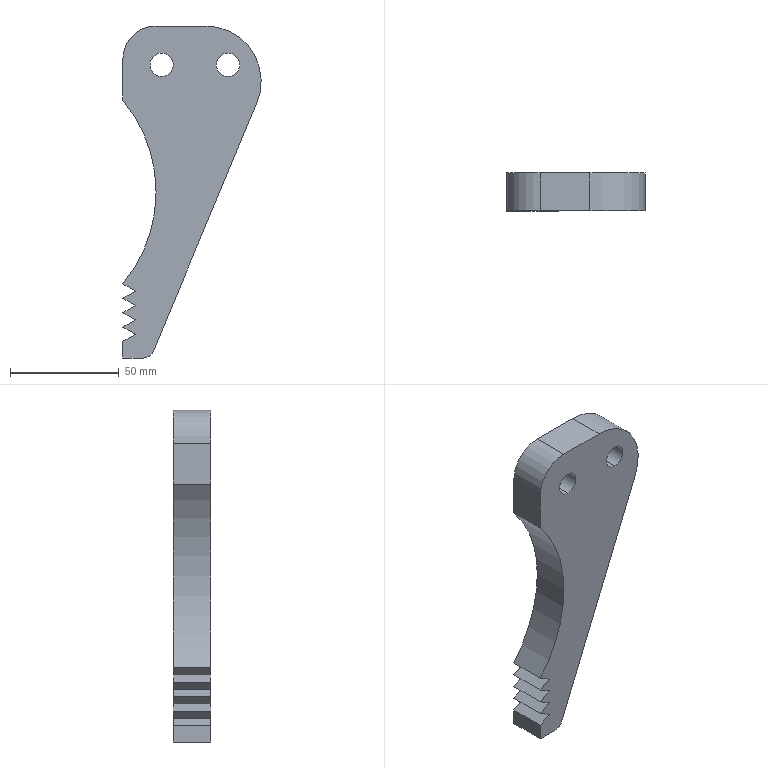Part | SolidWorks | features Fillet 3, ICE 2, Extrusion 1, Scale 1 | 1 solid | 23 faces | box 63.5 x 17.272 x 152.4 mm | volume 90763 mm3 | plane 15 | cylinder 8 | commonest cylinder face diameters 10.668 x4 10.16 x1 30.48 x1 50.8 x1 132.08 x1
STEP:
#1=CARTESIAN_POINT('',(48.26,0.,-23.114));
#2=VERTEX_POINT('',#1);
#3=CARTESIAN_POINT('',(48.26,0.,-12.446));
#4=VERTEX_POINT('',#3);
#5=CARTESIAN_POINT('',(48.26,0.,-17.78));
#6=DIRECTION('',(0.,1.,0.));
#7=DIRECTION('',(0.,0.,1.));
#8=AXIS2_PLACEMENT_3D('',#5,#6,#7);
#9=CIRCLE('',#8,5.334);
#10=EDGE_CURVE('',#2,#4,#9,.T.);
#11=ORIENTED_EDGE('',*,*,#10,.F.);
#12=CARTESIAN_POINT('',(48.26,17.272,-23.114));
#13=VERTEX_POINT('',#12);
#14=CARTESIAN_POINT('',(48.26,-20.828,-23.114));
#15=DIRECTION('',(0.,1.,0.));
#16=VECTOR('',#15,1000.);
#17=LINE('',#14,#16);
#18=EDGE_CURVE('',#2,#13,#17,.T.);
#19=ORIENTED_EDGE('',*,*,#18,.T.);
#20=CARTESIAN_POINT('',(48.26,17.272,-12.446));
#21=VERTEX_POINT('',#20);
#22=CARTESIAN_POINT('',(48.26,17.272,-17.78));
#23=DIRECTION('',(0.,1.,0.));
#24=DIRECTION('',(0.,0.,1.));
#25=AXIS2_PLACEMENT_3D('',#22,#23,#24);
#26=CIRCLE('',#25,5.334);
#27=EDGE_CURVE('',#13,#21,#26,.T.);
#28=ORIENTED_EDGE('',*,*,#27,.T.);
#29=CARTESIAN_POINT('',(48.26,-20.828,-12.446));
#30=DIRECTION('',(0.,1.,0.));
#31=VECTOR('',#30,1000.);
#32=LINE('',#29,#31);
#33=EDGE_CURVE('',#4,#21,#32,.T.);
#34=ORIENTED_EDGE('',*,*,#33,.F.);
#35=EDGE_LOOP('',(#11,#19,#28,#34));
#36=FACE_OUTER_BOUND('',#35,.T.);
#37=CARTESIAN_POINT('',(48.26,-20.828,-17.78));
#38=DIRECTION('',(0.,1.,0.));
#39=DIRECTION('',(0.,0.,1.));
#40=AXIS2_PLACEMENT_3D('',#37,#38,#39);
#41=CYLINDRICAL_SURFACE('',#40,5.334);
#42=ADVANCED_FACE('',(#36),#41,.F.);
#43=CARTESIAN_POINT('',(17.78,0.,-23.114));
#44=VERTEX_POINT('',#43);
#45=CARTESIAN_POINT('',(17.78,0.,-12.446));
#46=VERTEX_POINT('',#45);
#47=CARTESIAN_POINT('',(17.78,0.,-17.78));
#48=DIRECTION('',(0.,1.,0.));
#49=DIRECTION('',(0.,0.,1.));
#50=AXIS2_PLACEMENT_3D('',#47,#48,#49);
#51=CIRCLE('',#50,5.334);
#52=EDGE_CURVE('',#44,#46,#51,.T.);
#53=ORIENTED_EDGE('',*,*,#52,.F.);
#54=CARTESIAN_POINT('',(17.78,17.272,-23.114));
#55=VERTEX_POINT('',#54);
#56=CARTESIAN_POINT('',(17.78,-20.828,-23.114));
#57=DIRECTION('',(0.,1.,0.));
#58=VECTOR('',#57,1000.);
#59=LINE('',#56,#58);
#60=EDGE_CURVE('',#44,#55,#59,.T.);
#61=ORIENTED_EDGE('',*,*,#60,.T.);
#62=CARTESIAN_POINT('',(17.78,17.272,-12.446));
#63=VERTEX_POINT('',#62);
#64=CARTESIAN_POINT('',(17.78,17.272,-17.78));
#65=DIRECTION('',(0.,1.,0.));
#66=DIRECTION('',(0.,0.,1.));
#67=AXIS2_PLACEMENT_3D('',#64,#65,#66);
#68=CIRCLE('',#67,5.334);
#69=EDGE_CURVE('',#55,#63,#68,.T.);
#70=ORIENTED_EDGE('',*,*,#69,.T.);
#71=CARTESIAN_POINT('',(17.78,-20.828,-12.446));
#72=DIRECTION('',(0.,1.,0.));
#73=VECTOR('',#72,1000.);
#74=LINE('',#71,#73);
#75=EDGE_CURVE('',#46,#63,#74,.T.);
#76=ORIENTED_EDGE('',*,*,#75,.F.);
#77=EDGE_LOOP('',(#53,#61,#70,#76));
#78=FACE_OUTER_BOUND('',#77,.T.);
#79=CARTESIAN_POINT('',(17.78,-20.828,-17.78));
#80=DIRECTION('',(0.,1.,0.));
#81=DIRECTION('',(0.,0.,1.));
#82=AXIS2_PLACEMENT_3D('',#79,#80,#81);
#83=CYLINDRICAL_SURFACE('',#82,5.334);
#84=ADVANCED_FACE('',(#78),#83,.F.);
#85=CARTESIAN_POINT('',(0.,0.,-34.002));
#86=VERTEX_POINT('',#85);
#87=CARTESIAN_POINT('',(0.,0.,-15.24));
#88=VERTEX_POINT('',#87);
#89=CARTESIAN_POINT('',(0.,0.,0.));
#90=DIRECTION('',(0.,0.,1.));
#91=VECTOR('',#90,1000.);
#92=LINE('',#89,#91);
#93=EDGE_CURVE('',#86,#88,#92,.T.);
#94=ORIENTED_EDGE('',*,*,#93,.T.);
#95=CARTESIAN_POINT('',(0.,17.272,-15.24));
#96=VERTEX_POINT('',#95);
#97=CARTESIAN_POINT('',(0.,17.272,-15.24));
#98=DIRECTION('',(0.,1.,0.));
#99=VECTOR('',#98,1000.);
#100=LINE('',#97,#99);
#101=EDGE_CURVE('',#88,#96,#100,.T.);
#102=ORIENTED_EDGE('',*,*,#101,.T.);
#103=CARTESIAN_POINT('',(0.,17.272,-34.002));
#104=VERTEX_POINT('',#103);
#105=CARTESIAN_POINT('',(0.,17.272,0.));
#106=DIRECTION('',(0.,0.,1.));
#107=VECTOR('',#106,1000.);
#108=LINE('',#105,#107);
#109=EDGE_CURVE('',#104,#96,#108,.T.);
#110=ORIENTED_EDGE('',*,*,#109,.F.);
#111=CARTESIAN_POINT('',(0.,17.272,-34.002));
#112=DIRECTION('',(0.,-1.,0.));
#113=VECTOR('',#112,1000.);
#114=LINE('',#111,#113);
#115=EDGE_CURVE('',#104,#86,#114,.T.);
#116=ORIENTED_EDGE('',*,*,#115,.T.);
#117=EDGE_LOOP('',(#94,#102,#110,#116));
#118=FACE_OUTER_BOUND('',#117,.T.);
#119=CARTESIAN_POINT('',(0.,17.272,0.));
#120=DIRECTION('',(1.,0.,0.));
#121=DIRECTION('',(0.,0.,-1.));
#122=AXIS2_PLACEMENT_3D('',#119,#120,#121);
#123=PLANE('',#122);
#124=ADVANCED_FACE('',(#118),#123,.F.);
#125=CARTESIAN_POINT('',(15.24,17.272,0.));
#126=VERTEX_POINT('',#125);
#127=CARTESIAN_POINT('',(38.1,17.272,0.));
#128=VERTEX_POINT('',#127);
#129=CARTESIAN_POINT('',(0.,17.272,0.));
#130=DIRECTION('',(1.,0.,0.));
#131=VECTOR('',#130,1000.);
#132=LINE('',#129,#131);
#133=EDGE_CURVE('',#126,#128,#132,.T.);
#134=ORIENTED_EDGE('',*,*,#133,.F.);
#135=CARTESIAN_POINT('',(15.24,0.,0.));
#136=VERTEX_POINT('',#135);
#137=CARTESIAN_POINT('',(15.24,17.272,0.));
#138=DIRECTION('',(0.,-1.,0.));
#139=VECTOR('',#138,1000.);
#140=LINE('',#137,#139);
#141=EDGE_CURVE('',#126,#136,#140,.T.);
#142=ORIENTED_EDGE('',*,*,#141,.T.);
#143=CARTESIAN_POINT('',(38.1,0.,0.));
#144=VERTEX_POINT('',#143);
#145=CARTESIAN_POINT('',(0.,0.,0.));
#146=DIRECTION('',(1.,0.,0.));
#147=VECTOR('',#146,1000.);
#148=LINE('',#145,#147);
#149=EDGE_CURVE('',#136,#144,#148,.T.);
#150=ORIENTED_EDGE('',*,*,#149,.T.);
#151=CARTESIAN_POINT('',(38.1,17.272,0.));
#152=DIRECTION('',(0.,1.,0.));
#153=VECTOR('',#152,1000.);
#154=LINE('',#151,#153);
#155=EDGE_CURVE('',#144,#128,#154,.T.);
#156=ORIENTED_EDGE('',*,*,#155,.T.);
#157=EDGE_LOOP('',(#134,#142,#150,#156));
#158=FACE_OUTER_BOUND('',#157,.T.);
#159=CARTESIAN_POINT('',(0.,17.272,0.));
#160=DIRECTION('',(0.,0.,-1.));
#161=DIRECTION('',(-1.,0.,0.));
#162=AXIS2_PLACEMENT_3D('',#159,#160,#161);
#163=PLANE('',#162);
#164=ADVANCED_FACE('',(#158),#163,.F.);
#165=CARTESIAN_POINT('',(61.546,0.,-35.169));
#166=VERTEX_POINT('',#165);
#167=CARTESIAN_POINT('',(14.003,0.,-149.274));
#168=VERTEX_POINT('',#167);
#169=CARTESIAN_POINT('',(76.2,0.,0.));
#170=DIRECTION('',(-0.3846,0.,-0.9231));
#171=VECTOR('',#170,1000.);
#172=LINE('',#169,#171);
#173=EDGE_CURVE('',#166,#168,#172,.T.);
#174=ORIENTED_EDGE('',*,*,#173,.T.);
#175=CARTESIAN_POINT('',(14.003,17.272,-149.274));
#176=VERTEX_POINT('',#175);
#177=CARTESIAN_POINT('',(14.003,17.272,-149.274));
#178=DIRECTION('',(0.,1.,0.));
#179=VECTOR('',#178,1000.);
#180=LINE('',#177,#179);
#181=EDGE_CURVE('',#168,#176,#180,.T.);
#182=ORIENTED_EDGE('',*,*,#181,.T.);
#183=CARTESIAN_POINT('',(61.546,17.272,-35.169));
#184=VERTEX_POINT('',#183);
#185=CARTESIAN_POINT('',(76.2,17.272,0.));
#186=DIRECTION('',(-0.3846,0.,-0.9231));
#187=VECTOR('',#186,1000.);
#188=LINE('',#185,#187);
#189=EDGE_CURVE('',#184,#176,#188,.T.);
#190=ORIENTED_EDGE('',*,*,#189,.F.);
#191=CARTESIAN_POINT('',(61.546,17.272,-35.169));
#192=DIRECTION('',(0.,-1.,0.));
#193=VECTOR('',#192,1000.);
#194=LINE('',#191,#193);
#195=EDGE_CURVE('',#184,#166,#194,.T.);
#196=ORIENTED_EDGE('',*,*,#195,.T.);
#197=EDGE_LOOP('',(#174,#182,#190,#196));
#198=FACE_OUTER_BOUND('',#197,.T.);
#199=CARTESIAN_POINT('',(76.2,17.272,0.));
#200=DIRECTION('',(-0.9231,0.,0.3846));
#201=DIRECTION('',(0.3846,0.,0.9231));
#202=AXIS2_PLACEMENT_3D('',#199,#200,#201);
#203=PLANE('',#202);
#204=ADVANCED_FACE('',(#198),#203,.F.);
#205=CARTESIAN_POINT('',(9.313,17.272,-152.4));
#206=VERTEX_POINT('',#205);
#207=CARTESIAN_POINT('',(0.,17.272,-152.4));
#208=VERTEX_POINT('',#207);
#209=CARTESIAN_POINT('',(12.7,17.272,-152.4));
#210=DIRECTION('',(-1.,0.,0.));
#211=VECTOR('',#210,1000.);
#212=LINE('',#209,#211);
#213=EDGE_CURVE('',#206,#208,#212,.T.);
#214=ORIENTED_EDGE('',*,*,#213,.F.);
#215=CARTESIAN_POINT('',(9.313,0.,-152.4));
#216=VERTEX_POINT('',#215);
#217=CARTESIAN_POINT('',(9.313,17.272,-152.4));
#218=DIRECTION('',(0.,-1.,0.));
#219=VECTOR('',#218,1000.);
#220=LINE('',#217,#219);
#221=EDGE_CURVE('',#206,#216,#220,.T.);
#222=ORIENTED_EDGE('',*,*,#221,.T.);
#223=CARTESIAN_POINT('',(0.,0.,-152.4));
#224=VERTEX_POINT('',#223);
#225=CARTESIAN_POINT('',(12.7,0.,-152.4));
#226=DIRECTION('',(-1.,0.,0.));
#227=VECTOR('',#226,1000.);
#228=LINE('',#225,#227);
#229=EDGE_CURVE('',#216,#224,#228,.T.);
#230=ORIENTED_EDGE('',*,*,#229,.T.);
#231=CARTESIAN_POINT('',(0.,17.272,-152.4));
#232=DIRECTION('',(0.,-1.,0.));
#233=VECTOR('',#232,1000.);
#234=LINE('',#231,#233);
#235=EDGE_CURVE('',#208,#224,#234,.T.);
#236=ORIENTED_EDGE('',*,*,#235,.F.);
#237=EDGE_LOOP('',(#214,#222,#230,#236));
#238=FACE_OUTER_BOUND('',#237,.T.);
#239=CARTESIAN_POINT('',(12.7,17.272,-152.4));
#240=DIRECTION('',(0.,0.,1.));
#241=DIRECTION('',(1.,0.,0.));
#242=AXIS2_PLACEMENT_3D('',#239,#240,#241);
#243=PLANE('',#242);
#244=ADVANCED_FACE('',(#238),#243,.F.);
#245=CARTESIAN_POINT('',(0.,0.,-144.814));
#246=VERTEX_POINT('',#245);
#247=CARTESIAN_POINT('',(0.,0.,-152.4));
#248=DIRECTION('',(0.,0.,1.));
#249=VECTOR('',#248,1000.);
#250=LINE('',#247,#249);
#251=EDGE_CURVE('',#224,#246,#250,.T.);
#252=ORIENTED_EDGE('',*,*,#251,.T.);
#253=CARTESIAN_POINT('',(0.,17.272,-144.814));
#254=VERTEX_POINT('',#253);
#255=CARTESIAN_POINT('',(0.,0.,-144.814));
#256=DIRECTION('',(0.,1.,0.));
#257=VECTOR('',#256,1000.);
#258=LINE('',#255,#257);
#259=EDGE_CURVE('',#246,#254,#258,.T.);
#260=ORIENTED_EDGE('',*,*,#259,.T.);
#261=CARTESIAN_POINT('',(0.,17.272,-152.4));
#262=DIRECTION('',(0.,0.,1.));
#263=VECTOR('',#262,1000.);
#264=LINE('',#261,#263);
#265=EDGE_CURVE('',#208,#254,#264,.T.);
#266=ORIENTED_EDGE('',*,*,#265,.F.);
#267=ORIENTED_EDGE('',*,*,#235,.T.);
#268=EDGE_LOOP('',(#252,#260,#266,#267));
#269=FACE_OUTER_BOUND('',#268,.T.);
#270=CARTESIAN_POINT('',(0.,17.272,-152.4));
#271=DIRECTION('',(1.,0.,0.));
#272=DIRECTION('',(0.,0.,-1.));
#273=AXIS2_PLACEMENT_3D('',#270,#271,#272);
#274=PLANE('',#273);
#275=ADVANCED_FACE('',(#269),#274,.F.);
#276=CARTESIAN_POINT('',(0.,0.,-118.398));
#277=VERTEX_POINT('',#276);
#278=CARTESIAN_POINT('',(-50.8,0.,-76.2));
#279=DIRECTION('',(0.,-1.,0.));
#280=DIRECTION('',(0.,0.,1.));
#281=AXIS2_PLACEMENT_3D('',#278,#279,#280);
#282=CIRCLE('',#281,66.04);
#283=EDGE_CURVE('',#277,#86,#282,.T.);
#284=ORIENTED_EDGE('',*,*,#283,.T.);
#285=ORIENTED_EDGE('',*,*,#115,.F.);
#286=CARTESIAN_POINT('',(0.,17.272,-118.398));
#287=VERTEX_POINT('',#286);
#288=CARTESIAN_POINT('',(-50.8,17.272,-76.2));
#289=DIRECTION('',(0.,-1.,0.));
#290=DIRECTION('',(0.,0.,1.));
#291=AXIS2_PLACEMENT_3D('',#288,#289,#290);
#292=CIRCLE('',#291,66.04);
#293=EDGE_CURVE('',#287,#104,#292,.T.);
#294=ORIENTED_EDGE('',*,*,#293,.F.);
#295=CARTESIAN_POINT('',(0.,17.272,-118.398));
#296=DIRECTION('',(0.,-1.,0.));
#297=VECTOR('',#296,1000.);
#298=LINE('',#295,#297);
#299=EDGE_CURVE('',#287,#277,#298,.T.);
#300=ORIENTED_EDGE('',*,*,#299,.T.);
#301=EDGE_LOOP('',(#284,#285,#294,#300));
#302=FACE_OUTER_BOUND('',#301,.T.);
#303=CARTESIAN_POINT('',(-50.8,17.272,-76.2));
#304=DIRECTION('',(0.,-1.,0.));
#305=DIRECTION('',(0.,0.,-1.));
#306=AXIS2_PLACEMENT_3D('',#303,#304,#305);
#307=CYLINDRICAL_SURFACE('',#306,66.04);
#308=ADVANCED_FACE('',(#302),#307,.F.);
#309=CARTESIAN_POINT('',(0.,17.272,-138.21));
#310=VERTEX_POINT('',#309);
#311=CARTESIAN_POINT('',(5.719,17.272,-141.512));
#312=VERTEX_POINT('',#311);
#313=CARTESIAN_POINT('',(-59.847,17.272,-103.657));
#314=DIRECTION('',(0.866,0.,-0.5));
#315=VECTOR('',#314,1000.);
#316=LINE('',#313,#315);
#317=EDGE_CURVE('',#310,#312,#316,.T.);
#318=ORIENTED_EDGE('',*,*,#317,.F.);
#319=CARTESIAN_POINT('',(5.719,17.272,-134.908));
#320=VERTEX_POINT('',#319);
#321=CARTESIAN_POINT('',(59.847,17.272,-103.657));
#322=DIRECTION('',(-0.866,0.,-0.5));
#323=VECTOR('',#322,1000.);
#324=LINE('',#321,#323);
#325=EDGE_CURVE('',#320,#310,#324,.T.);
#326=ORIENTED_EDGE('',*,*,#325,.F.);
#327=CARTESIAN_POINT('',(0.,17.272,-131.606));
#328=VERTEX_POINT('',#327);
#329=CARTESIAN_POINT('',(-56.987,17.272,-98.704));
#330=DIRECTION('',(0.866,0.,-0.5));
#331=VECTOR('',#330,1000.);
#332=LINE('',#329,#331);
#333=EDGE_CURVE('',#328,#320,#332,.T.);
#334=ORIENTED_EDGE('',*,*,#333,.F.);
#335=CARTESIAN_POINT('',(5.719,17.272,-128.304));
#336=VERTEX_POINT('',#335);
#337=CARTESIAN_POINT('',(56.987,17.272,-98.704));
#338=DIRECTION('',(-0.866,0.,-0.5));
#339=VECTOR('',#338,1000.);
#340=LINE('',#337,#339);
#341=EDGE_CURVE('',#336,#328,#340,.T.);
#342=ORIENTED_EDGE('',*,*,#341,.F.);
#343=CARTESIAN_POINT('',(0.,17.272,-125.002));
#344=VERTEX_POINT('',#343);
#345=CARTESIAN_POINT('',(-54.127,17.272,-93.751));
#346=DIRECTION('',(0.866,0.,-0.5));
#347=VECTOR('',#346,1000.);
#348=LINE('',#345,#347);
#349=EDGE_CURVE('',#344,#336,#348,.T.);
#350=ORIENTED_EDGE('',*,*,#349,.F.);
#351=CARTESIAN_POINT('',(5.719,17.272,-121.7));
#352=VERTEX_POINT('',#351);
#353=CARTESIAN_POINT('',(54.127,17.272,-93.751));
#354=DIRECTION('',(-0.866,0.,-0.5));
#355=VECTOR('',#354,1000.);
#356=LINE('',#353,#355);
#357=EDGE_CURVE('',#352,#344,#356,.T.);
#358=ORIENTED_EDGE('',*,*,#357,.F.);
#359=CARTESIAN_POINT('',(-51.268,17.272,-88.798));
#360=DIRECTION('',(0.866,0.,-0.5));
#361=VECTOR('',#360,1000.);
#362=LINE('',#359,#361);
#363=EDGE_CURVE('',#287,#352,#362,.T.);
#364=ORIENTED_EDGE('',*,*,#363,.F.);
#365=ORIENTED_EDGE('',*,*,#293,.T.);
#366=ORIENTED_EDGE('',*,*,#109,.T.);
#367=CARTESIAN_POINT('',(15.24,17.272,-15.24));
#368=DIRECTION('',(0.,1.,0.));
#369=DIRECTION('',(0.,0.,1.));
#370=AXIS2_PLACEMENT_3D('',#367,#368,#369);
#371=CIRCLE('',#370,15.24);
#372=EDGE_CURVE('',#96,#126,#371,.T.);
#373=ORIENTED_EDGE('',*,*,#372,.T.);
#374=ORIENTED_EDGE('',*,*,#133,.T.);
#375=CARTESIAN_POINT('',(38.1,17.272,-25.4));
#376=DIRECTION('',(0.,1.,0.));
#377=DIRECTION('',(0.,0.,1.));
#378=AXIS2_PLACEMENT_3D('',#375,#376,#377);
#379=CIRCLE('',#378,25.4);
#380=EDGE_CURVE('',#128,#184,#379,.T.);
#381=ORIENTED_EDGE('',*,*,#380,.T.);
#382=ORIENTED_EDGE('',*,*,#189,.T.);
#383=CARTESIAN_POINT('',(9.313,17.272,-147.32));
#384=DIRECTION('',(0.,1.,0.));
#385=DIRECTION('',(0.,0.,1.));
#386=AXIS2_PLACEMENT_3D('',#383,#384,#385);
#387=CIRCLE('',#386,5.08);
#388=EDGE_CURVE('',#176,#206,#387,.T.);
#389=ORIENTED_EDGE('',*,*,#388,.T.);
#390=ORIENTED_EDGE('',*,*,#213,.T.);
#391=ORIENTED_EDGE('',*,*,#265,.T.);
#392=CARTESIAN_POINT('',(62.706,17.272,-108.61));
#393=DIRECTION('',(-0.866,0.,-0.5));
#394=VECTOR('',#393,1000.);
#395=LINE('',#392,#394);
#396=EDGE_CURVE('',#312,#254,#395,.T.);
#397=ORIENTED_EDGE('',*,*,#396,.F.);
#398=EDGE_LOOP('',(#318,#326,#334,#342,#350,#358,#364,#365,#366,#373,#374,#381,#382,#389,#390,#391,#397));
#399=FACE_OUTER_BOUND('',#398,.T.);
#400=CARTESIAN_POINT('',(48.26,17.272,-17.78));
#401=DIRECTION('',(0.,1.,0.));
#402=DIRECTION('',(0.,0.,1.));
#403=AXIS2_PLACEMENT_3D('',#400,#401,#402);
#404=CIRCLE('',#403,5.334);
#405=EDGE_CURVE('',#21,#13,#404,.T.);
#406=ORIENTED_EDGE('',*,*,#405,.F.);
#407=ORIENTED_EDGE('',*,*,#27,.F.);
#408=EDGE_LOOP('',(#406,#407));
#409=FACE_BOUND('',#408,.T.);
#410=CARTESIAN_POINT('',(17.78,17.272,-17.78));
#411=DIRECTION('',(0.,1.,0.));
#412=DIRECTION('',(0.,0.,1.));
#413=AXIS2_PLACEMENT_3D('',#410,#411,#412);
#414=CIRCLE('',#413,5.334);
#415=EDGE_CURVE('',#63,#55,#414,.T.);
#416=ORIENTED_EDGE('',*,*,#415,.F.);
#417=ORIENTED_EDGE('',*,*,#69,.F.);
#418=EDGE_LOOP('',(#416,#417));
#419=FACE_BOUND('',#418,.T.);
#420=CARTESIAN_POINT('',(-50.8,17.272,-76.2));
#421=DIRECTION('',(0.,1.,0.));
#422=DIRECTION('',(0.,0.,1.));
#423=AXIS2_PLACEMENT_3D('',#420,#421,#422);
#424=PLANE('',#423);
#425=ADVANCED_FACE('',(#399,#409,#419),#424,.T.);
#426=CARTESIAN_POINT('',(48.26,0.,-17.78));
#427=DIRECTION('',(0.,1.,0.));
#428=DIRECTION('',(0.,0.,1.));
#429=AXIS2_PLACEMENT_3D('',#426,#427,#428);
#430=CIRCLE('',#429,5.334);
#431=EDGE_CURVE('',#4,#2,#430,.T.);
#432=ORIENTED_EDGE('',*,*,#431,.T.);
#433=ORIENTED_EDGE('',*,*,#10,.T.);
#434=EDGE_LOOP('',(#432,#433));
#435=FACE_BOUND('',#434,.T.);
#436=CARTESIAN_POINT('',(17.78,0.,-17.78));
#437=DIRECTION('',(0.,1.,0.));
#438=DIRECTION('',(0.,0.,1.));
#439=AXIS2_PLACEMENT_3D('',#436,#437,#438);
#440=CIRCLE('',#439,5.334);
#441=EDGE_CURVE('',#46,#44,#440,.T.);
#442=ORIENTED_EDGE('',*,*,#441,.T.);
#443=ORIENTED_EDGE('',*,*,#52,.T.);
#444=EDGE_LOOP('',(#442,#443));
#445=FACE_BOUND('',#444,.T.);
#446=CARTESIAN_POINT('',(5.719,0.,-134.908));
#447=VERTEX_POINT('',#446);
#448=CARTESIAN_POINT('',(0.,0.,-138.21));
#449=VERTEX_POINT('',#448);
#450=CARTESIAN_POINT('',(59.847,0.,-103.657));
#451=DIRECTION('',(-0.866,0.,-0.5));
#452=VECTOR('',#451,1000.);
#453=LINE('',#450,#452);
#454=EDGE_CURVE('',#447,#449,#453,.T.);
#455=ORIENTED_EDGE('',*,*,#454,.T.);
#456=CARTESIAN_POINT('',(5.719,0.,-141.512));
#457=VERTEX_POINT('',#456);
#458=CARTESIAN_POINT('',(-59.847,0.,-103.657));
#459=DIRECTION('',(0.866,0.,-0.5));
#460=VECTOR('',#459,1000.);
#461=LINE('',#458,#460);
#462=EDGE_CURVE('',#449,#457,#461,.T.);
#463=ORIENTED_EDGE('',*,*,#462,.T.);
#464=CARTESIAN_POINT('',(62.706,0.,-108.61));
#465=DIRECTION('',(-0.866,0.,-0.5));
#466=VECTOR('',#465,1000.);
#467=LINE('',#464,#466);
#468=EDGE_CURVE('',#457,#246,#467,.T.);
#469=ORIENTED_EDGE('',*,*,#468,.T.);
#470=ORIENTED_EDGE('',*,*,#251,.F.);
#471=ORIENTED_EDGE('',*,*,#229,.F.);
#472=CARTESIAN_POINT('',(9.313,0.,-147.32));
#473=DIRECTION('',(0.,-1.,0.));
#474=DIRECTION('',(0.,0.,1.));
#475=AXIS2_PLACEMENT_3D('',#472,#473,#474);
#476=CIRCLE('',#475,5.08);
#477=EDGE_CURVE('',#216,#168,#476,.T.);
#478=ORIENTED_EDGE('',*,*,#477,.T.);
#479=ORIENTED_EDGE('',*,*,#173,.F.);
#480=CARTESIAN_POINT('',(38.1,0.,-25.4));
#481=DIRECTION('',(0.,-1.,0.));
#482=DIRECTION('',(0.,0.,1.));
#483=AXIS2_PLACEMENT_3D('',#480,#481,#482);
#484=CIRCLE('',#483,25.4);
#485=EDGE_CURVE('',#166,#144,#484,.T.);
#486=ORIENTED_EDGE('',*,*,#485,.T.);
#487=ORIENTED_EDGE('',*,*,#149,.F.);
#488=CARTESIAN_POINT('',(15.24,0.,-15.24));
#489=DIRECTION('',(0.,-1.,0.));
#490=DIRECTION('',(0.,0.,1.));
#491=AXIS2_PLACEMENT_3D('',#488,#489,#490);
#492=CIRCLE('',#491,15.24);
#493=EDGE_CURVE('',#136,#88,#492,.T.);
#494=ORIENTED_EDGE('',*,*,#493,.T.);
#495=ORIENTED_EDGE('',*,*,#93,.F.);
#496=ORIENTED_EDGE('',*,*,#283,.F.);
#497=CARTESIAN_POINT('',(5.719,0.,-121.7));
#498=VERTEX_POINT('',#497);
#499=CARTESIAN_POINT('',(-51.268,0.,-88.798));
#500=DIRECTION('',(0.866,0.,-0.5));
#501=VECTOR('',#500,1000.);
#502=LINE('',#499,#501);
#503=EDGE_CURVE('',#277,#498,#502,.T.);
#504=ORIENTED_EDGE('',*,*,#503,.T.);
#505=CARTESIAN_POINT('',(0.,0.,-125.002));
#506=VERTEX_POINT('',#505);
#507=CARTESIAN_POINT('',(54.127,0.,-93.751));
#508=DIRECTION('',(-0.866,0.,-0.5));
#509=VECTOR('',#508,1000.);
#510=LINE('',#507,#509);
#511=EDGE_CURVE('',#498,#506,#510,.T.);
#512=ORIENTED_EDGE('',*,*,#511,.T.);
#513=CARTESIAN_POINT('',(5.719,0.,-128.304));
#514=VERTEX_POINT('',#513);
#515=CARTESIAN_POINT('',(-54.127,0.,-93.751));
#516=DIRECTION('',(0.866,0.,-0.5));
#517=VECTOR('',#516,1000.);
#518=LINE('',#515,#517);
#519=EDGE_CURVE('',#506,#514,#518,.T.);
#520=ORIENTED_EDGE('',*,*,#519,.T.);
#521=CARTESIAN_POINT('',(0.,0.,-131.606));
#522=VERTEX_POINT('',#521);
#523=CARTESIAN_POINT('',(56.987,0.,-98.704));
#524=DIRECTION('',(-0.866,0.,-0.5));
#525=VECTOR('',#524,1000.);
#526=LINE('',#523,#525);
#527=EDGE_CURVE('',#514,#522,#526,.T.);
#528=ORIENTED_EDGE('',*,*,#527,.T.);
#529=CARTESIAN_POINT('',(-56.987,0.,-98.704));
#530=DIRECTION('',(0.866,0.,-0.5));
#531=VECTOR('',#530,1000.);
#532=LINE('',#529,#531);
#533=EDGE_CURVE('',#522,#447,#532,.T.);
#534=ORIENTED_EDGE('',*,*,#533,.T.);
#535=EDGE_LOOP('',(#455,#463,#469,#470,#471,#478,#479,#486,#487,#494,#495,#496,#504,#512,#520,#528,#534));
#536=FACE_OUTER_BOUND('',#535,.T.);
#537=CARTESIAN_POINT('',(-50.8,0.,-76.2));
#538=DIRECTION('',(0.,1.,0.));
#539=DIRECTION('',(0.,0.,1.));
#540=AXIS2_PLACEMENT_3D('',#537,#538,#539);
#541=PLANE('',#540);
#542=ADVANCED_FACE('',(#435,#445,#536),#541,.F.);
#543=ORIENTED_EDGE('',*,*,#60,.F.);
#544=ORIENTED_EDGE('',*,*,#441,.F.);
#545=ORIENTED_EDGE('',*,*,#75,.T.);
#546=ORIENTED_EDGE('',*,*,#415,.T.);
#547=EDGE_LOOP('',(#543,#544,#545,#546));
#548=FACE_OUTER_BOUND('',#547,.T.);
#549=CARTESIAN_POINT('',(17.78,-20.828,-17.78));
#550=DIRECTION('',(0.,1.,0.));
#551=DIRECTION('',(0.,0.,1.));
#552=AXIS2_PLACEMENT_3D('',#549,#550,#551);
#553=CYLINDRICAL_SURFACE('',#552,5.334);
#554=ADVANCED_FACE('',(#548),#553,.F.);
#555=ORIENTED_EDGE('',*,*,#18,.F.);
#556=ORIENTED_EDGE('',*,*,#431,.F.);
#557=ORIENTED_EDGE('',*,*,#33,.T.);
#558=ORIENTED_EDGE('',*,*,#405,.T.);
#559=EDGE_LOOP('',(#555,#556,#557,#558));
#560=FACE_OUTER_BOUND('',#559,.T.);
#561=CARTESIAN_POINT('',(48.26,-20.828,-17.78));
#562=DIRECTION('',(0.,1.,0.));
#563=DIRECTION('',(0.,0.,1.));
#564=AXIS2_PLACEMENT_3D('',#561,#562,#563);
#565=CYLINDRICAL_SURFACE('',#564,5.334);
#566=ADVANCED_FACE('',(#560),#565,.F.);
#567=ORIENTED_EDGE('',*,*,#380,.F.);
#568=ORIENTED_EDGE('',*,*,#155,.F.);
#569=ORIENTED_EDGE('',*,*,#485,.F.);
#570=ORIENTED_EDGE('',*,*,#195,.F.);
#571=EDGE_LOOP('',(#567,#568,#569,#570));
#572=FACE_OUTER_BOUND('',#571,.T.);
#573=CARTESIAN_POINT('',(38.1,17.272,-25.4));
#574=DIRECTION('',(0.,-1.,0.));
#575=DIRECTION('',(0.,0.,-1.));
#576=AXIS2_PLACEMENT_3D('',#573,#574,#575);
#577=CYLINDRICAL_SURFACE('',#576,25.4);
#578=ADVANCED_FACE('',(#572),#577,.T.);
#579=ORIENTED_EDGE('',*,*,#388,.F.);
#580=ORIENTED_EDGE('',*,*,#181,.F.);
#581=ORIENTED_EDGE('',*,*,#477,.F.);
#582=ORIENTED_EDGE('',*,*,#221,.F.);
#583=EDGE_LOOP('',(#579,#580,#581,#582));
#584=FACE_OUTER_BOUND('',#583,.T.);
#585=CARTESIAN_POINT('',(9.313,17.272,-147.32));
#586=DIRECTION('',(0.,-1.,0.));
#587=DIRECTION('',(0.,0.,-1.));
#588=AXIS2_PLACEMENT_3D('',#585,#586,#587);
#589=CYLINDRICAL_SURFACE('',#588,5.08);
#590=ADVANCED_FACE('',(#584),#589,.T.);
#591=ORIENTED_EDGE('',*,*,#372,.F.);
#592=ORIENTED_EDGE('',*,*,#101,.F.);
#593=ORIENTED_EDGE('',*,*,#493,.F.);
#594=ORIENTED_EDGE('',*,*,#141,.F.);
#595=EDGE_LOOP('',(#591,#592,#593,#594));
#596=FACE_OUTER_BOUND('',#595,.T.);
#597=CARTESIAN_POINT('',(15.24,17.272,-15.24));
#598=DIRECTION('',(0.,-1.,0.));
#599=DIRECTION('',(0.,0.,-1.));
#600=AXIS2_PLACEMENT_3D('',#597,#598,#599);
#601=CYLINDRICAL_SURFACE('',#600,15.24);
#602=ADVANCED_FACE('',(#596),#601,.T.);
#603=ORIENTED_EDGE('',*,*,#363,.T.);
#604=CARTESIAN_POINT('',(5.719,0.,-121.7));
#605=DIRECTION('',(0.,1.,0.));
#606=VECTOR('',#605,1000.);
#607=LINE('',#604,#606);
#608=EDGE_CURVE('',#498,#352,#607,.T.);
#609=ORIENTED_EDGE('',*,*,#608,.F.);
#610=ORIENTED_EDGE('',*,*,#503,.F.);
#611=ORIENTED_EDGE('',*,*,#299,.F.);
#612=EDGE_LOOP('',(#603,#609,#610,#611));
#613=FACE_OUTER_BOUND('',#612,.T.);
#614=CARTESIAN_POINT('',(-51.268,0.,-88.798));
#615=DIRECTION('',(0.5,0.,0.866));
#616=DIRECTION('',(0.866,0.,-0.5));
#617=AXIS2_PLACEMENT_3D('',#614,#615,#616);
#618=PLANE('',#617);
#619=ADVANCED_FACE('',(#613),#618,.F.);
#620=ORIENTED_EDGE('',*,*,#357,.T.);
#621=CARTESIAN_POINT('',(0.,0.,-125.002));
#622=DIRECTION('',(0.,1.,0.));
#623=VECTOR('',#622,1000.);
#624=LINE('',#621,#623);
#625=EDGE_CURVE('',#506,#344,#624,.T.);
#626=ORIENTED_EDGE('',*,*,#625,.F.);
#627=ORIENTED_EDGE('',*,*,#511,.F.);
#628=ORIENTED_EDGE('',*,*,#608,.T.);
#629=EDGE_LOOP('',(#620,#626,#627,#628));
#630=FACE_OUTER_BOUND('',#629,.T.);
#631=CARTESIAN_POINT('',(54.127,0.,-93.751));
#632=DIRECTION('',(0.5,0.,-0.866));
#633=DIRECTION('',(-0.866,0.,-0.5));
#634=AXIS2_PLACEMENT_3D('',#631,#632,#633);
#635=PLANE('',#634);
#636=ADVANCED_FACE('',(#630),#635,.F.);
#637=ORIENTED_EDGE('',*,*,#349,.T.);
#638=CARTESIAN_POINT('',(5.719,0.,-128.304));
#639=DIRECTION('',(0.,1.,0.));
#640=VECTOR('',#639,1000.);
#641=LINE('',#638,#640);
#642=EDGE_CURVE('',#514,#336,#641,.T.);
#643=ORIENTED_EDGE('',*,*,#642,.F.);
#644=ORIENTED_EDGE('',*,*,#519,.F.);
#645=ORIENTED_EDGE('',*,*,#625,.T.);
#646=EDGE_LOOP('',(#637,#643,#644,#645));
#647=FACE_OUTER_BOUND('',#646,.T.);
#648=CARTESIAN_POINT('',(-54.127,0.,-93.751));
#649=DIRECTION('',(0.5,0.,0.866));
#650=DIRECTION('',(0.866,0.,-0.5));
#651=AXIS2_PLACEMENT_3D('',#648,#649,#650);
#652=PLANE('',#651);
#653=ADVANCED_FACE('',(#647),#652,.F.);
#654=ORIENTED_EDGE('',*,*,#341,.T.);
#655=CARTESIAN_POINT('',(0.,0.,-131.606));
#656=DIRECTION('',(0.,1.,0.));
#657=VECTOR('',#656,1000.);
#658=LINE('',#655,#657);
#659=EDGE_CURVE('',#522,#328,#658,.T.);
#660=ORIENTED_EDGE('',*,*,#659,.F.);
#661=ORIENTED_EDGE('',*,*,#527,.F.);
#662=ORIENTED_EDGE('',*,*,#642,.T.);
#663=EDGE_LOOP('',(#654,#660,#661,#662));
#664=FACE_OUTER_BOUND('',#663,.T.);
#665=CARTESIAN_POINT('',(56.987,0.,-98.704));
#666=DIRECTION('',(0.5,0.,-0.866));
#667=DIRECTION('',(-0.866,0.,-0.5));
#668=AXIS2_PLACEMENT_3D('',#665,#666,#667);
#669=PLANE('',#668);
#670=ADVANCED_FACE('',(#664),#669,.F.);
#671=ORIENTED_EDGE('',*,*,#333,.T.);
#672=CARTESIAN_POINT('',(5.719,0.,-134.908));
#673=DIRECTION('',(0.,1.,0.));
#674=VECTOR('',#673,1000.);
#675=LINE('',#672,#674);
#676=EDGE_CURVE('',#447,#320,#675,.T.);
#677=ORIENTED_EDGE('',*,*,#676,.F.);
#678=ORIENTED_EDGE('',*,*,#533,.F.);
#679=ORIENTED_EDGE('',*,*,#659,.T.);
#680=EDGE_LOOP('',(#671,#677,#678,#679));
#681=FACE_OUTER_BOUND('',#680,.T.);
#682=CARTESIAN_POINT('',(-56.987,0.,-98.704));
#683=DIRECTION('',(0.5,0.,0.866));
#684=DIRECTION('',(0.866,0.,-0.5));
#685=AXIS2_PLACEMENT_3D('',#682,#683,#684);
#686=PLANE('',#685);
#687=ADVANCED_FACE('',(#681),#686,.F.);
#688=ORIENTED_EDGE('',*,*,#325,.T.);
#689=CARTESIAN_POINT('',(0.,0.,-138.21));
#690=DIRECTION('',(0.,1.,0.));
#691=VECTOR('',#690,1000.);
#692=LINE('',#689,#691);
#693=EDGE_CURVE('',#449,#310,#692,.T.);
#694=ORIENTED_EDGE('',*,*,#693,.F.);
#695=ORIENTED_EDGE('',*,*,#454,.F.);
#696=ORIENTED_EDGE('',*,*,#676,.T.);
#697=EDGE_LOOP('',(#688,#694,#695,#696));
#698=FACE_OUTER_BOUND('',#697,.T.);
#699=CARTESIAN_POINT('',(59.847,0.,-103.657));
#700=DIRECTION('',(0.5,0.,-0.866));
#701=DIRECTION('',(-0.866,0.,-0.5));
#702=AXIS2_PLACEMENT_3D('',#699,#700,#701);
#703=PLANE('',#702);
#704=ADVANCED_FACE('',(#698),#703,.F.);
#705=ORIENTED_EDGE('',*,*,#317,.T.);
#706=CARTESIAN_POINT('',(5.719,0.,-141.512));
#707=DIRECTION('',(0.,1.,0.));
#708=VECTOR('',#707,1000.);
#709=LINE('',#706,#708);
#710=EDGE_CURVE('',#457,#312,#709,.T.);
#711=ORIENTED_EDGE('',*,*,#710,.F.);
#712=ORIENTED_EDGE('',*,*,#462,.F.);
#713=ORIENTED_EDGE('',*,*,#693,.T.);
#714=EDGE_LOOP('',(#705,#711,#712,#713));
#715=FACE_OUTER_BOUND('',#714,.T.);
#716=CARTESIAN_POINT('',(-59.847,0.,-103.657));
#717=DIRECTION('',(0.5,0.,0.866));
#718=DIRECTION('',(0.866,0.,-0.5));
#719=AXIS2_PLACEMENT_3D('',#716,#717,#718);
#720=PLANE('',#719);
#721=ADVANCED_FACE('',(#715),#720,.F.);
#722=ORIENTED_EDGE('',*,*,#396,.T.);
#723=ORIENTED_EDGE('',*,*,#259,.F.);
#724=ORIENTED_EDGE('',*,*,#468,.F.);
#725=ORIENTED_EDGE('',*,*,#710,.T.);
#726=EDGE_LOOP('',(#722,#723,#724,#725));
#727=FACE_OUTER_BOUND('',#726,.T.);
#728=CARTESIAN_POINT('',(62.706,0.,-108.61));
#729=DIRECTION('',(0.5,0.,-0.866));
#730=DIRECTION('',(-0.866,0.,-0.5));
#731=AXIS2_PLACEMENT_3D('',#728,#729,#730);
#732=PLANE('',#731);
#733=ADVANCED_FACE('',(#727),#732,.F.);
#734=CLOSED_SHELL('',(#42,#84,#124,#164,#204,#244,#275,#308,#425,#542,#554,#566,#578,#590,#602,#619,#636,#653,#670,#687,#704,#721,#733));
#735=MANIFOLD_SOLID_BREP('',#734);
#736=CARTESIAN_POINT('',(0.,0.,0.));
#737=DIRECTION('',(0.,0.,1.));
#738=DIRECTION('',(1.,0.,0.));
#739=AXIS2_PLACEMENT_3D('',#736,#737,#738);
#740=(LENGTH_UNIT()NAMED_UNIT(*)SI_UNIT(.MILLI.,.METRE.));
#741=UNCERTAINTY_MEASURE_WITH_UNIT(LENGTH_MEASURE(0.00001),#740,'','');
#742=(NAMED_UNIT(*)PLANE_ANGLE_UNIT()SI_UNIT($,.RADIAN.));
#743=(NAMED_UNIT(*)SI_UNIT($,.STERADIAN.)SOLID_ANGLE_UNIT());
#744=(GEOMETRIC_REPRESENTATION_CONTEXT(3)GLOBAL_UNCERTAINTY_ASSIGNED_CONTEXT((#741))GLOBAL_UNIT_ASSIGNED_CONTEXT((#740,#742,#743))REPRESENTATION_CONTEXT('',''));
#745=ADVANCED_BREP_SHAPE_REPRESENTATION('',(#735,#739),#744);